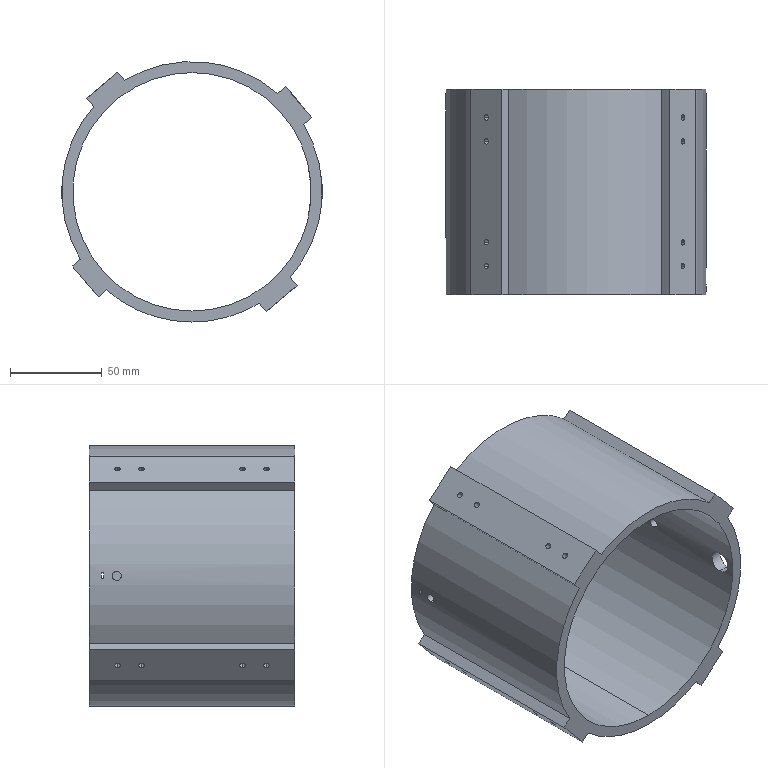Part | SolidWorks | features ICE 7, CirPattern 1, RefAxis 1, Revolution 1 | 1 solid | 85 faces | box 142 x 112 x 142 mm | volume 337681 mm3 | cylinder 51 | plane 34 | commonest cylinder face diameters 3 x32 1.2 x6 142 x5 5 x4 12 x2 130 x2